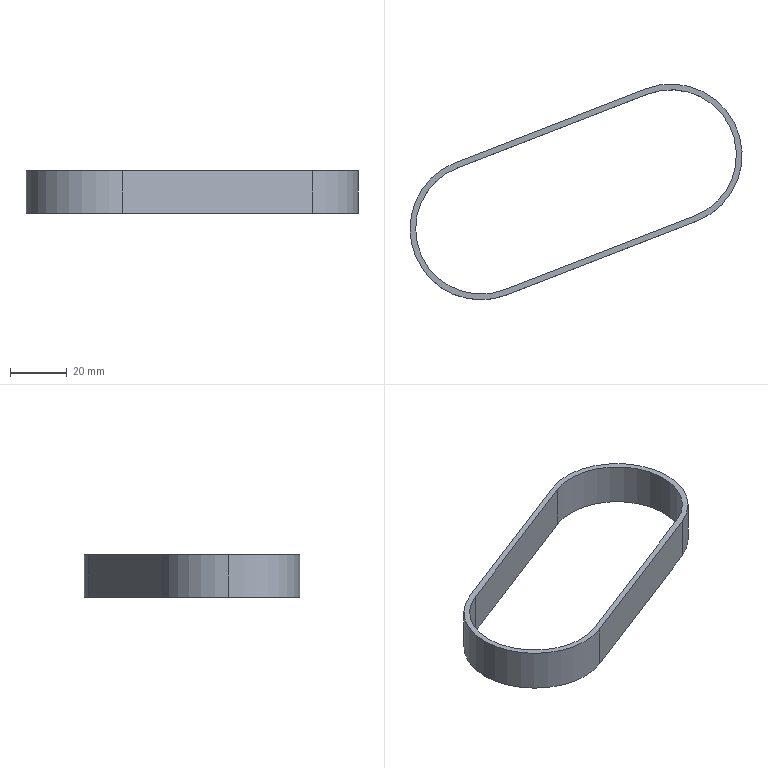Part | SolidWorks | features BaseBody 1 | 1 solid | 12 faces | box 117 x 76 x 15 mm | volume 8836 mm3 | cylinder 6 | plane 6 | commonest cylinder face diameters 46 x3 50 x3
STEP:
#1=CARTESIAN_POINT('',(-75.321,-4.558,7.5));
#2=VERTEX_POINT('',#1);
#3=CARTESIAN_POINT('',(-90.,-26.,7.5));
#4=VERTEX_POINT('',#3);
#5=CARTESIAN_POINT('',(-67.,-26.,7.5));
#6=DIRECTION('',(0.,0.,1.));
#7=DIRECTION('',(1.,0.,0.));
#8=AXIS2_PLACEMENT_3D('',#5,#6,#7);
#9=CIRCLE('',#8,23.);
#10=EDGE_CURVE('',#2,#4,#9,.T.);
#11=ORIENTED_EDGE('',*,*,#10,.T.);
#12=CARTESIAN_POINT('',(-90.,-26.,-7.5));
#13=VERTEX_POINT('',#12);
#14=CARTESIAN_POINT('',(-90.,-26.,7.5));
#15=DIRECTION('',(0.,0.,-1.));
#16=VECTOR('',#15,1000.);
#17=LINE('',#14,#16);
#18=EDGE_CURVE('',#4,#13,#17,.T.);
#19=ORIENTED_EDGE('',*,*,#18,.T.);
#20=CARTESIAN_POINT('',(-75.321,-4.558,-7.5));
#21=VERTEX_POINT('',#20);
#22=CARTESIAN_POINT('',(-67.,-26.,-7.5));
#23=DIRECTION('',(0.,0.,1.));
#24=DIRECTION('',(1.,0.,0.));
#25=AXIS2_PLACEMENT_3D('',#22,#23,#24);
#26=CIRCLE('',#25,23.);
#27=EDGE_CURVE('',#21,#13,#26,.T.);
#28=ORIENTED_EDGE('',*,*,#27,.F.);
#29=CARTESIAN_POINT('',(-75.321,-4.558,7.5));
#30=DIRECTION('',(0.,0.,-1.));
#31=VECTOR('',#30,1000.);
#32=LINE('',#29,#31);
#33=EDGE_CURVE('',#2,#21,#32,.T.);
#34=ORIENTED_EDGE('',*,*,#33,.F.);
#35=EDGE_LOOP('',(#11,#19,#28,#34));
#36=FACE_OUTER_BOUND('',#35,.T.);
#37=CARTESIAN_POINT('',(-67.,-26.,7.5));
#38=DIRECTION('',(0.,0.,-1.));
#39=DIRECTION('',(-1.,0.,0.));
#40=AXIS2_PLACEMENT_3D('',#37,#38,#39);
#41=CYLINDRICAL_SURFACE('',#40,23.);
#42=ADVANCED_FACE('',(#36),#41,.F.);
#43=CARTESIAN_POINT('',(-92.,-26.,7.5));
#44=VERTEX_POINT('',#43);
#45=CARTESIAN_POINT('',(-57.956,-49.307,7.5));
#46=VERTEX_POINT('',#45);
#47=CARTESIAN_POINT('',(-67.,-26.,7.5));
#48=DIRECTION('',(0.,0.,1.));
#49=DIRECTION('',(1.,0.,0.));
#50=AXIS2_PLACEMENT_3D('',#47,#48,#49);
#51=CIRCLE('',#50,25.);
#52=EDGE_CURVE('',#44,#46,#51,.T.);
#53=ORIENTED_EDGE('',*,*,#52,.F.);
#54=CARTESIAN_POINT('',(-92.,-26.,-7.5));
#55=VERTEX_POINT('',#54);
#56=CARTESIAN_POINT('',(-92.,-26.,7.5));
#57=DIRECTION('',(0.,0.,-1.));
#58=VECTOR('',#57,1000.);
#59=LINE('',#56,#58);
#60=EDGE_CURVE('',#44,#55,#59,.T.);
#61=ORIENTED_EDGE('',*,*,#60,.T.);
#62=CARTESIAN_POINT('',(-57.956,-49.307,-7.5));
#63=VERTEX_POINT('',#62);
#64=CARTESIAN_POINT('',(-67.,-26.,-7.5));
#65=DIRECTION('',(0.,0.,1.));
#66=DIRECTION('',(1.,0.,0.));
#67=AXIS2_PLACEMENT_3D('',#64,#65,#66);
#68=CIRCLE('',#67,25.);
#69=EDGE_CURVE('',#55,#63,#68,.T.);
#70=ORIENTED_EDGE('',*,*,#69,.T.);
#71=CARTESIAN_POINT('',(-57.956,-49.307,7.5));
#72=DIRECTION('',(0.,0.,-1.));
#73=VECTOR('',#72,1000.);
#74=LINE('',#71,#73);
#75=EDGE_CURVE('',#46,#63,#74,.T.);
#76=ORIENTED_EDGE('',*,*,#75,.F.);
#77=EDGE_LOOP('',(#53,#61,#70,#76));
#78=FACE_OUTER_BOUND('',#77,.T.);
#79=CARTESIAN_POINT('',(-67.,-26.,7.5));
#80=DIRECTION('',(0.,0.,-1.));
#81=DIRECTION('',(-1.,0.,0.));
#82=AXIS2_PLACEMENT_3D('',#79,#80,#81);
#83=CYLINDRICAL_SURFACE('',#82,25.);
#84=ADVANCED_FACE('',(#78),#83,.T.);
#85=CARTESIAN_POINT('',(-58.679,-47.442,-7.5));
#86=VERTEX_POINT('',#85);
#87=CARTESIAN_POINT('',(8.321,-21.442,-7.5));
#88=VERTEX_POINT('',#87);
#89=CARTESIAN_POINT('',(8.321,-21.442,-7.5));
#90=DIRECTION('',(0.9323,0.3618,0.));
#91=VECTOR('',#90,1000.);
#92=LINE('',#89,#91);
#93=EDGE_CURVE('',#86,#88,#92,.T.);
#94=ORIENTED_EDGE('',*,*,#93,.F.);
#95=CARTESIAN_POINT('',(-58.679,-47.442,7.5));
#96=VERTEX_POINT('',#95);
#97=CARTESIAN_POINT('',(-58.679,-47.442,7.5));
#98=DIRECTION('',(0.,0.,-1.));
#99=VECTOR('',#98,1000.);
#100=LINE('',#97,#99);
#101=EDGE_CURVE('',#96,#86,#100,.T.);
#102=ORIENTED_EDGE('',*,*,#101,.F.);
#103=CARTESIAN_POINT('',(8.321,-21.442,7.5));
#104=VERTEX_POINT('',#103);
#105=CARTESIAN_POINT('',(8.321,-21.442,7.5));
#106=DIRECTION('',(0.9323,0.3618,0.));
#107=VECTOR('',#106,1000.);
#108=LINE('',#105,#107);
#109=EDGE_CURVE('',#96,#104,#108,.T.);
#110=ORIENTED_EDGE('',*,*,#109,.T.);
#111=CARTESIAN_POINT('',(8.321,-21.442,7.5));
#112=DIRECTION('',(0.,0.,-1.));
#113=VECTOR('',#112,1000.);
#114=LINE('',#111,#113);
#115=EDGE_CURVE('',#104,#88,#114,.T.);
#116=ORIENTED_EDGE('',*,*,#115,.T.);
#117=EDGE_LOOP('',(#94,#102,#110,#116));
#118=FACE_OUTER_BOUND('',#117,.T.);
#119=CARTESIAN_POINT('',(8.321,-21.442,7.5));
#120=DIRECTION('',(-0.3618,0.9323,0.));
#121=DIRECTION('',(0.,0.,1.));
#122=AXIS2_PLACEMENT_3D('',#119,#120,#121);
#123=PLANE('',#122);
#124=ADVANCED_FACE('',(#118),#123,.T.);
#125=CARTESIAN_POINT('',(-8.321,21.442,-7.5));
#126=VERTEX_POINT('',#125);
#127=CARTESIAN_POINT('',(-8.321,21.442,-7.5));
#128=DIRECTION('',(-0.9323,-0.3618,0.));
#129=VECTOR('',#128,1000.);
#130=LINE('',#127,#129);
#131=EDGE_CURVE('',#126,#21,#130,.T.);
#132=ORIENTED_EDGE('',*,*,#131,.F.);
#133=CARTESIAN_POINT('',(-8.321,21.442,7.5));
#134=VERTEX_POINT('',#133);
#135=CARTESIAN_POINT('',(-8.321,21.442,7.5));
#136=DIRECTION('',(0.,0.,-1.));
#137=VECTOR('',#136,1000.);
#138=LINE('',#135,#137);
#139=EDGE_CURVE('',#134,#126,#138,.T.);
#140=ORIENTED_EDGE('',*,*,#139,.F.);
#141=CARTESIAN_POINT('',(-8.321,21.442,7.5));
#142=DIRECTION('',(-0.9323,-0.3618,0.));
#143=VECTOR('',#142,1000.);
#144=LINE('',#141,#143);
#145=EDGE_CURVE('',#134,#2,#144,.T.);
#146=ORIENTED_EDGE('',*,*,#145,.T.);
#147=ORIENTED_EDGE('',*,*,#33,.T.);
#148=EDGE_LOOP('',(#132,#140,#146,#147));
#149=FACE_OUTER_BOUND('',#148,.T.);
#150=CARTESIAN_POINT('',(-8.321,21.442,7.5));
#151=DIRECTION('',(0.3618,-0.9323,0.));
#152=DIRECTION('',(0.,0.,-1.));
#153=AXIS2_PLACEMENT_3D('',#150,#151,#152);
#154=PLANE('',#153);
#155=ADVANCED_FACE('',(#149),#154,.T.);
#156=CARTESIAN_POINT('',(0.,0.,-7.5));
#157=DIRECTION('',(0.,0.,1.));
#158=DIRECTION('',(1.,0.,0.));
#159=AXIS2_PLACEMENT_3D('',#156,#157,#158);
#160=CIRCLE('',#159,23.);
#161=EDGE_CURVE('',#88,#126,#160,.T.);
#162=ORIENTED_EDGE('',*,*,#161,.F.);
#163=ORIENTED_EDGE('',*,*,#115,.F.);
#164=CARTESIAN_POINT('',(0.,0.,7.5));
#165=DIRECTION('',(0.,0.,1.));
#166=DIRECTION('',(1.,0.,0.));
#167=AXIS2_PLACEMENT_3D('',#164,#165,#166);
#168=CIRCLE('',#167,23.);
#169=EDGE_CURVE('',#104,#134,#168,.T.);
#170=ORIENTED_EDGE('',*,*,#169,.T.);
#171=ORIENTED_EDGE('',*,*,#139,.T.);
#172=EDGE_LOOP('',(#162,#163,#170,#171));
#173=FACE_OUTER_BOUND('',#172,.T.);
#174=CARTESIAN_POINT('',(0.,0.,7.5));
#175=DIRECTION('',(0.,0.,-1.));
#176=DIRECTION('',(-1.,0.,0.));
#177=AXIS2_PLACEMENT_3D('',#174,#175,#176);
#178=CYLINDRICAL_SURFACE('',#177,23.);
#179=ADVANCED_FACE('',(#173),#178,.F.);
#180=CARTESIAN_POINT('',(9.044,-23.307,-7.5));
#181=VERTEX_POINT('',#180);
#182=CARTESIAN_POINT('',(9.044,-23.307,-7.5));
#183=DIRECTION('',(0.9323,0.3618,0.));
#184=VECTOR('',#183,1000.);
#185=LINE('',#182,#184);
#186=EDGE_CURVE('',#63,#181,#185,.T.);
#187=ORIENTED_EDGE('',*,*,#186,.T.);
#188=CARTESIAN_POINT('',(9.044,-23.307,7.5));
#189=VERTEX_POINT('',#188);
#190=CARTESIAN_POINT('',(9.044,-23.307,7.5));
#191=DIRECTION('',(0.,0.,-1.));
#192=VECTOR('',#191,1000.);
#193=LINE('',#190,#192);
#194=EDGE_CURVE('',#189,#181,#193,.T.);
#195=ORIENTED_EDGE('',*,*,#194,.F.);
#196=CARTESIAN_POINT('',(9.044,-23.307,7.5));
#197=DIRECTION('',(0.9323,0.3618,0.));
#198=VECTOR('',#197,1000.);
#199=LINE('',#196,#198);
#200=EDGE_CURVE('',#46,#189,#199,.T.);
#201=ORIENTED_EDGE('',*,*,#200,.F.);
#202=ORIENTED_EDGE('',*,*,#75,.T.);
#203=EDGE_LOOP('',(#187,#195,#201,#202));
#204=FACE_OUTER_BOUND('',#203,.T.);
#205=CARTESIAN_POINT('',(9.044,-23.307,7.5));
#206=DIRECTION('',(-0.3618,0.9323,0.));
#207=DIRECTION('',(0.,0.,1.));
#208=AXIS2_PLACEMENT_3D('',#205,#206,#207);
#209=PLANE('',#208);
#210=ADVANCED_FACE('',(#204),#209,.F.);
#211=CARTESIAN_POINT('',(-9.044,23.307,-7.5));
#212=VERTEX_POINT('',#211);
#213=CARTESIAN_POINT('',(-76.044,-2.693,-7.5));
#214=VERTEX_POINT('',#213);
#215=CARTESIAN_POINT('',(-9.044,23.307,-7.5));
#216=DIRECTION('',(-0.9323,-0.3618,0.));
#217=VECTOR('',#216,1000.);
#218=LINE('',#215,#217);
#219=EDGE_CURVE('',#212,#214,#218,.T.);
#220=ORIENTED_EDGE('',*,*,#219,.T.);
#221=CARTESIAN_POINT('',(-76.044,-2.693,7.5));
#222=VERTEX_POINT('',#221);
#223=CARTESIAN_POINT('',(-76.044,-2.693,7.5));
#224=DIRECTION('',(0.,0.,-1.));
#225=VECTOR('',#224,1000.);
#226=LINE('',#223,#225);
#227=EDGE_CURVE('',#222,#214,#226,.T.);
#228=ORIENTED_EDGE('',*,*,#227,.F.);
#229=CARTESIAN_POINT('',(-9.044,23.307,7.5));
#230=VERTEX_POINT('',#229);
#231=CARTESIAN_POINT('',(-9.044,23.307,7.5));
#232=DIRECTION('',(-0.9323,-0.3618,0.));
#233=VECTOR('',#232,1000.);
#234=LINE('',#231,#233);
#235=EDGE_CURVE('',#230,#222,#234,.T.);
#236=ORIENTED_EDGE('',*,*,#235,.F.);
#237=CARTESIAN_POINT('',(-9.044,23.307,7.5));
#238=DIRECTION('',(0.,0.,-1.));
#239=VECTOR('',#238,1000.);
#240=LINE('',#237,#239);
#241=EDGE_CURVE('',#230,#212,#240,.T.);
#242=ORIENTED_EDGE('',*,*,#241,.T.);
#243=EDGE_LOOP('',(#220,#228,#236,#242));
#244=FACE_OUTER_BOUND('',#243,.T.);
#245=CARTESIAN_POINT('',(-9.044,23.307,7.5));
#246=DIRECTION('',(0.3618,-0.9323,0.));
#247=DIRECTION('',(0.,0.,-1.));
#248=AXIS2_PLACEMENT_3D('',#245,#246,#247);
#249=PLANE('',#248);
#250=ADVANCED_FACE('',(#244),#249,.F.);
#251=CARTESIAN_POINT('',(0.,0.,-7.5));
#252=DIRECTION('',(0.,0.,1.));
#253=DIRECTION('',(1.,0.,0.));
#254=AXIS2_PLACEMENT_3D('',#251,#252,#253);
#255=CIRCLE('',#254,25.);
#256=EDGE_CURVE('',#181,#212,#255,.T.);
#257=ORIENTED_EDGE('',*,*,#256,.T.);
#258=ORIENTED_EDGE('',*,*,#241,.F.);
#259=CARTESIAN_POINT('',(0.,0.,7.5));
#260=DIRECTION('',(0.,0.,1.));
#261=DIRECTION('',(1.,0.,0.));
#262=AXIS2_PLACEMENT_3D('',#259,#260,#261);
#263=CIRCLE('',#262,25.);
#264=EDGE_CURVE('',#189,#230,#263,.T.);
#265=ORIENTED_EDGE('',*,*,#264,.F.);
#266=ORIENTED_EDGE('',*,*,#194,.T.);
#267=EDGE_LOOP('',(#257,#258,#265,#266));
#268=FACE_OUTER_BOUND('',#267,.T.);
#269=CARTESIAN_POINT('',(0.,0.,7.5));
#270=DIRECTION('',(0.,0.,-1.));
#271=DIRECTION('',(-1.,0.,0.));
#272=AXIS2_PLACEMENT_3D('',#269,#270,#271);
#273=CYLINDRICAL_SURFACE('',#272,25.);
#274=ADVANCED_FACE('',(#268),#273,.T.);
#275=ORIENTED_EDGE('',*,*,#161,.T.);
#276=ORIENTED_EDGE('',*,*,#131,.T.);
#277=ORIENTED_EDGE('',*,*,#27,.T.);
#278=CARTESIAN_POINT('',(-67.,-26.,-7.5));
#279=DIRECTION('',(0.,0.,1.));
#280=DIRECTION('',(1.,0.,0.));
#281=AXIS2_PLACEMENT_3D('',#278,#279,#280);
#282=CIRCLE('',#281,23.);
#283=EDGE_CURVE('',#13,#86,#282,.T.);
#284=ORIENTED_EDGE('',*,*,#283,.T.);
#285=ORIENTED_EDGE('',*,*,#93,.T.);
#286=EDGE_LOOP('',(#275,#276,#277,#284,#285));
#287=FACE_BOUND('',#286,.T.);
#288=ORIENTED_EDGE('',*,*,#256,.F.);
#289=ORIENTED_EDGE('',*,*,#186,.F.);
#290=ORIENTED_EDGE('',*,*,#69,.F.);
#291=CARTESIAN_POINT('',(-67.,-26.,-7.5));
#292=DIRECTION('',(0.,0.,1.));
#293=DIRECTION('',(1.,0.,0.));
#294=AXIS2_PLACEMENT_3D('',#291,#292,#293);
#295=CIRCLE('',#294,25.);
#296=EDGE_CURVE('',#214,#55,#295,.T.);
#297=ORIENTED_EDGE('',*,*,#296,.F.);
#298=ORIENTED_EDGE('',*,*,#219,.F.);
#299=EDGE_LOOP('',(#288,#289,#290,#297,#298));
#300=FACE_OUTER_BOUND('',#299,.T.);
#301=CARTESIAN_POINT('',(0.,0.,-7.5));
#302=DIRECTION('',(0.,0.,1.));
#303=DIRECTION('',(1.,0.,0.));
#304=AXIS2_PLACEMENT_3D('',#301,#302,#303);
#305=PLANE('',#304);
#306=ADVANCED_FACE('',(#287,#300),#305,.F.);
#307=ORIENTED_EDGE('',*,*,#145,.F.);
#308=ORIENTED_EDGE('',*,*,#169,.F.);
#309=ORIENTED_EDGE('',*,*,#109,.F.);
#310=CARTESIAN_POINT('',(-67.,-26.,7.5));
#311=DIRECTION('',(0.,0.,1.));
#312=DIRECTION('',(1.,0.,0.));
#313=AXIS2_PLACEMENT_3D('',#310,#311,#312);
#314=CIRCLE('',#313,23.);
#315=EDGE_CURVE('',#4,#96,#314,.T.);
#316=ORIENTED_EDGE('',*,*,#315,.F.);
#317=ORIENTED_EDGE('',*,*,#10,.F.);
#318=EDGE_LOOP('',(#307,#308,#309,#316,#317));
#319=FACE_BOUND('',#318,.T.);
#320=ORIENTED_EDGE('',*,*,#264,.T.);
#321=ORIENTED_EDGE('',*,*,#235,.T.);
#322=CARTESIAN_POINT('',(-67.,-26.,7.5));
#323=DIRECTION('',(0.,0.,1.));
#324=DIRECTION('',(1.,0.,0.));
#325=AXIS2_PLACEMENT_3D('',#322,#323,#324);
#326=CIRCLE('',#325,25.);
#327=EDGE_CURVE('',#222,#44,#326,.T.);
#328=ORIENTED_EDGE('',*,*,#327,.T.);
#329=ORIENTED_EDGE('',*,*,#52,.T.);
#330=ORIENTED_EDGE('',*,*,#200,.T.);
#331=EDGE_LOOP('',(#320,#321,#328,#329,#330));
#332=FACE_OUTER_BOUND('',#331,.T.);
#333=CARTESIAN_POINT('',(0.,0.,7.5));
#334=DIRECTION('',(0.,0.,1.));
#335=DIRECTION('',(1.,0.,0.));
#336=AXIS2_PLACEMENT_3D('',#333,#334,#335);
#337=PLANE('',#336);
#338=ADVANCED_FACE('',(#319,#332),#337,.T.);
#339=ORIENTED_EDGE('',*,*,#60,.F.);
#340=ORIENTED_EDGE('',*,*,#327,.F.);
#341=ORIENTED_EDGE('',*,*,#227,.T.);
#342=ORIENTED_EDGE('',*,*,#296,.T.);
#343=EDGE_LOOP('',(#339,#340,#341,#342));
#344=FACE_OUTER_BOUND('',#343,.T.);
#345=CARTESIAN_POINT('',(-67.,-26.,7.5));
#346=DIRECTION('',(0.,0.,-1.));
#347=DIRECTION('',(-1.,0.,0.));
#348=AXIS2_PLACEMENT_3D('',#345,#346,#347);
#349=CYLINDRICAL_SURFACE('',#348,25.);
#350=ADVANCED_FACE('',(#344),#349,.T.);
#351=ORIENTED_EDGE('',*,*,#18,.F.);
#352=ORIENTED_EDGE('',*,*,#315,.T.);
#353=ORIENTED_EDGE('',*,*,#101,.T.);
#354=ORIENTED_EDGE('',*,*,#283,.F.);
#355=EDGE_LOOP('',(#351,#352,#353,#354));
#356=FACE_OUTER_BOUND('',#355,.T.);
#357=CARTESIAN_POINT('',(-67.,-26.,7.5));
#358=DIRECTION('',(0.,0.,-1.));
#359=DIRECTION('',(-1.,0.,0.));
#360=AXIS2_PLACEMENT_3D('',#357,#358,#359);
#361=CYLINDRICAL_SURFACE('',#360,23.);
#362=ADVANCED_FACE('',(#356),#361,.F.);
#363=CLOSED_SHELL('',(#42,#84,#124,#155,#179,#210,#250,#274,#306,#338,#350,#362));
#364=MANIFOLD_SOLID_BREP('',#363);
#365=CARTESIAN_POINT('',(0.,0.,0.));
#366=DIRECTION('',(0.,0.,1.));
#367=DIRECTION('',(1.,0.,0.));
#368=AXIS2_PLACEMENT_3D('',#365,#366,#367);
#369=(LENGTH_UNIT()NAMED_UNIT(*)SI_UNIT(.MILLI.,.METRE.));
#370=UNCERTAINTY_MEASURE_WITH_UNIT(LENGTH_MEASURE(0.00001),#369,'','');
#371=(NAMED_UNIT(*)PLANE_ANGLE_UNIT()SI_UNIT($,.RADIAN.));
#372=(NAMED_UNIT(*)SI_UNIT($,.STERADIAN.)SOLID_ANGLE_UNIT());
#373=(GEOMETRIC_REPRESENTATION_CONTEXT(3)GLOBAL_UNCERTAINTY_ASSIGNED_CONTEXT((#370))GLOBAL_UNIT_ASSIGNED_CONTEXT((#369,#371,#372))REPRESENTATION_CONTEXT('',''));
#374=ADVANCED_BREP_SHAPE_REPRESENTATION('',(#364,#368),#373);